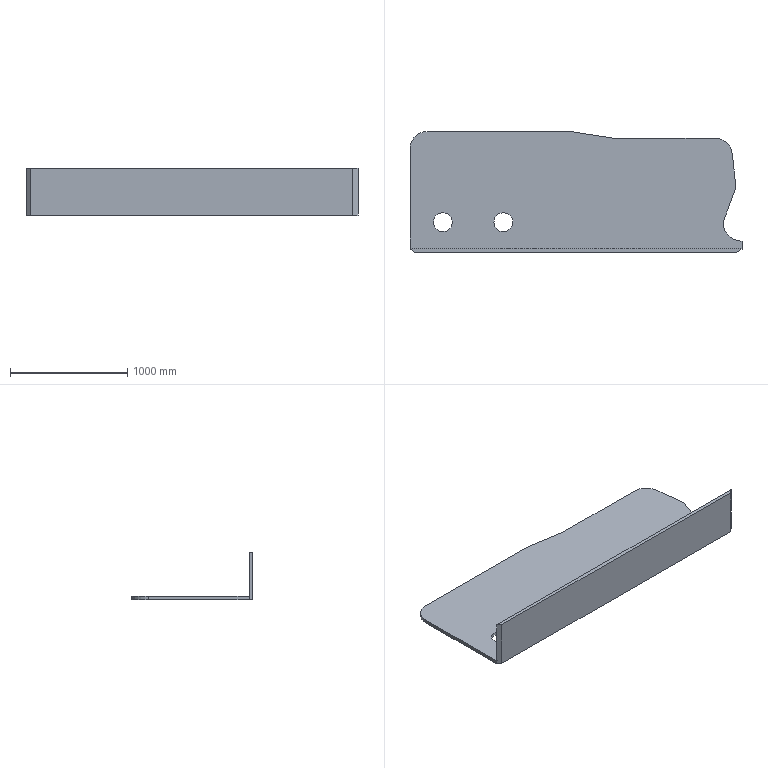Part | NX | features 掩护梁侧护板右 2 | 1 solid | 24 faces | box 2828 x 1030 x 405 mm | volume 109386503 mm3 | plane 18 | cylinder 6 | commonest cylinder face diameters 160.33 x2 291.509 x2 250.37 x1 322.604 x1
STEP:
#1=CARTESIAN_POINT('',(-541.636,-260.046,-750.));
#2=VERTEX_POINT('',#1);
#3=CARTESIAN_POINT('',(-621.801,-260.046,-750.));
#4=DIRECTION('',(0.,0.,1.));
#5=DIRECTION('',(1.,0.,0.));
#6=AXIS2_PLACEMENT_3D('',#3,#4,#5);
#7=CIRCLE('',#6,80.165);
#8=EDGE_CURVE('',#2,#2,#7,.T.);
#9=ORIENTED_EDGE('',*,*,#8,.F.);
#10=EDGE_LOOP('',(#9));
#11=FACE_BOUND('',#10,.T.);
#12=CARTESIAN_POINT('',(-1056.636,-260.046,-750.));
#13=VERTEX_POINT('',#12);
#14=CARTESIAN_POINT('',(-1136.801,-260.046,-750.));
#15=DIRECTION('',(0.,0.,1.));
#16=DIRECTION('',(1.,0.,0.));
#17=AXIS2_PLACEMENT_3D('',#14,#15,#16);
#18=CIRCLE('',#17,80.165);
#19=EDGE_CURVE('',#13,#13,#18,.T.);
#20=ORIENTED_EDGE('',*,*,#19,.F.);
#21=EDGE_LOOP('',(#20));
#22=FACE_BOUND('',#21,.T.);
#23=CARTESIAN_POINT('',(-1416.65,-488.395,-750.));
#24=VERTEX_POINT('',#23);
#25=CARTESIAN_POINT('',(1410.992,-488.395,-750.));
#26=VERTEX_POINT('',#25);
#27=CARTESIAN_POINT('',(1410.992,-488.395,-750.));
#28=DIRECTION('',(1.,0.,0.));
#29=VECTOR('',#28,1000.);
#30=LINE('',#27,#29);
#31=EDGE_CURVE('',#24,#26,#30,.T.);
#32=ORIENTED_EDGE('',*,*,#31,.T.);
#33=CARTESIAN_POINT('',(1410.992,-421.348,-750.));
#34=VERTEX_POINT('',#33);
#35=CARTESIAN_POINT('',(1410.992,-488.395,-750.));
#36=DIRECTION('',(0.,1.,0.));
#37=VECTOR('',#36,1000.);
#38=LINE('',#35,#37);
#39=EDGE_CURVE('',#26,#34,#38,.T.);
#40=ORIENTED_EDGE('',*,*,#39,.T.);
#41=CARTESIAN_POINT('',(1249.69,-260.046,-750.));
#42=VERTEX_POINT('',#41);
#43=CARTESIAN_POINT('',(1410.992,-260.046,-750.));
#44=DIRECTION('',(0.,0.,-1.));
#45=DIRECTION('',(1.,0.,0.));
#46=AXIS2_PLACEMENT_3D('',#43,#44,#45);
#47=CIRCLE('',#46,161.302);
#48=EDGE_CURVE('',#34,#42,#47,.T.);
#49=ORIENTED_EDGE('',*,*,#48,.T.);
#50=CARTESIAN_POINT('',(1359.76,36.697,-750.));
#51=VERTEX_POINT('',#50);
#52=CARTESIAN_POINT('',(1249.69,-260.046,-750.));
#53=DIRECTION('',(0.3478,0.9376,0.));
#54=VECTOR('',#53,1000.);
#55=LINE('',#52,#54);
#56=EDGE_CURVE('',#42,#51,#55,.T.);
#57=ORIENTED_EDGE('',*,*,#56,.T.);
#58=CARTESIAN_POINT('',(1327.809,324.481,-750.));
#59=VERTEX_POINT('',#58);
#60=CARTESIAN_POINT('',(1359.76,36.697,-750.));
#61=DIRECTION('',(-0.1103,0.9939,0.));
#62=VECTOR('',#61,1000.);
#63=LINE('',#60,#62);
#64=EDGE_CURVE('',#51,#59,#63,.T.);
#65=ORIENTED_EDGE('',*,*,#64,.T.);
#66=CARTESIAN_POINT('',(1182.944,454.152,-750.));
#67=VERTEX_POINT('',#66);
#68=CARTESIAN_POINT('',(1182.944,308.397,-750.));
#69=DIRECTION('',(0.,0.,1.));
#70=DIRECTION('',(1.,0.,0.));
#71=AXIS2_PLACEMENT_3D('',#68,#69,#70);
#72=CIRCLE('',#71,145.755);
#73=EDGE_CURVE('',#59,#67,#72,.T.);
#74=ORIENTED_EDGE('',*,*,#73,.T.);
#75=CARTESIAN_POINT('',(324.663,454.152,-750.));
#76=VERTEX_POINT('',#75);
#77=CARTESIAN_POINT('',(935.041,454.152,-750.));
#78=DIRECTION('',(-1.,0.,0.));
#79=VECTOR('',#78,1000.);
#80=LINE('',#77,#79);
#81=EDGE_CURVE('',#67,#76,#80,.T.);
#82=ORIENTED_EDGE('',*,*,#81,.T.);
#83=CARTESIAN_POINT('',(-51.414,512.454,-750.));
#84=VERTEX_POINT('',#83);
#85=CARTESIAN_POINT('',(324.663,454.152,-750.));
#86=DIRECTION('',(-0.9882,0.1532,0.));
#87=VECTOR('',#86,1000.);
#88=LINE('',#85,#87);
#89=EDGE_CURVE('',#76,#84,#88,.T.);
#90=ORIENTED_EDGE('',*,*,#89,.T.);
#91=CARTESIAN_POINT('',(-1270.895,512.454,-750.));
#92=VERTEX_POINT('',#91);
#93=CARTESIAN_POINT('',(-51.414,512.454,-750.));
#94=DIRECTION('',(-1.,0.,0.));
#95=VECTOR('',#94,1000.);
#96=LINE('',#93,#95);
#97=EDGE_CURVE('',#84,#92,#96,.T.);
#98=ORIENTED_EDGE('',*,*,#97,.T.);
#99=CARTESIAN_POINT('',(-1416.65,366.699,-750.));
#100=VERTEX_POINT('',#99);
#101=CARTESIAN_POINT('',(-1270.895,366.699,-750.));
#102=DIRECTION('',(0.,0.,1.));
#103=DIRECTION('',(1.,0.,0.));
#104=AXIS2_PLACEMENT_3D('',#101,#102,#103);
#105=CIRCLE('',#104,145.755);
#106=EDGE_CURVE('',#92,#100,#105,.T.);
#107=ORIENTED_EDGE('',*,*,#106,.T.);
#108=CARTESIAN_POINT('',(-1416.65,366.699,-750.));
#109=DIRECTION('',(0.,-1.,0.));
#110=VECTOR('',#109,1000.);
#111=LINE('',#108,#110);
#112=EDGE_CURVE('',#100,#24,#111,.T.);
#113=ORIENTED_EDGE('',*,*,#112,.T.);
#114=EDGE_LOOP('',(#32,#40,#49,#57,#65,#74,#82,#90,#98,#107,#113));
#115=FACE_BOUND('',#114,.T.);
#116=CARTESIAN_POINT('',(-1270.895,366.699,-750.));
#117=DIRECTION('',(0.,0.,-1.));
#118=DIRECTION('',(1.,0.,0.));
#119=AXIS2_PLACEMENT_3D('',#116,#117,#118);
#120=PLANE('',#119);
#121=ADVANCED_FACE('',(#11,#22,#115),#120,.F.);
#122=CARTESIAN_POINT('',(1410.992,-488.395,-775.));
#123=VERTEX_POINT('',#122);
#124=CARTESIAN_POINT('',(1410.992,-421.348,-775.));
#125=VERTEX_POINT('',#124);
#126=CARTESIAN_POINT('',(1410.992,-488.395,-775.));
#127=DIRECTION('',(0.,1.,0.));
#128=VECTOR('',#127,1000.);
#129=LINE('',#126,#128);
#130=EDGE_CURVE('',#123,#125,#129,.T.);
#131=ORIENTED_EDGE('',*,*,#130,.T.);
#132=CARTESIAN_POINT('',(1410.992,-421.348,-780.));
#133=DIRECTION('',(0.,0.,1.));
#134=VECTOR('',#133,1000.);
#135=LINE('',#132,#134);
#136=EDGE_CURVE('',#125,#34,#135,.T.);
#137=ORIENTED_EDGE('',*,*,#136,.T.);
#138=ORIENTED_EDGE('',*,*,#39,.F.);
#139=CARTESIAN_POINT('',(1410.992,-488.395,-780.));
#140=DIRECTION('',(0.,0.,1.));
#141=VECTOR('',#140,1000.);
#142=LINE('',#139,#141);
#143=EDGE_CURVE('',#123,#26,#142,.T.);
#144=ORIENTED_EDGE('',*,*,#143,.F.);
#145=EDGE_LOOP('',(#131,#137,#138,#144));
#146=FACE_BOUND('',#145,.T.);
#147=CARTESIAN_POINT('',(1410.992,-488.395,-780.));
#148=DIRECTION('',(-1.,0.,0.));
#149=DIRECTION('',(0.,-1.,0.));
#150=AXIS2_PLACEMENT_3D('',#147,#148,#149);
#151=PLANE('',#150);
#152=ADVANCED_FACE('',(#146),#151,.F.);
#153=CARTESIAN_POINT('',(1249.69,-260.046,-775.));
#154=VERTEX_POINT('',#153);
#155=CARTESIAN_POINT('',(1410.992,-260.046,-775.));
#156=DIRECTION('',(0.,0.,-1.));
#157=DIRECTION('',(1.,0.,0.));
#158=AXIS2_PLACEMENT_3D('',#155,#156,#157);
#159=CIRCLE('',#158,161.302);
#160=EDGE_CURVE('',#125,#154,#159,.T.);
#161=ORIENTED_EDGE('',*,*,#160,.T.);
#162=CARTESIAN_POINT('',(1249.69,-260.046,-780.));
#163=DIRECTION('',(0.,0.,1.));
#164=VECTOR('',#163,1000.);
#165=LINE('',#162,#164);
#166=EDGE_CURVE('',#154,#42,#165,.T.);
#167=ORIENTED_EDGE('',*,*,#166,.T.);
#168=ORIENTED_EDGE('',*,*,#48,.F.);
#169=ORIENTED_EDGE('',*,*,#136,.F.);
#170=EDGE_LOOP('',(#161,#167,#168,#169));
#171=FACE_BOUND('',#170,.T.);
#172=CARTESIAN_POINT('',(1410.992,-260.046,-780.));
#173=DIRECTION('',(0.,0.,1.));
#174=DIRECTION('',(-1.,0.,0.));
#175=AXIS2_PLACEMENT_3D('',#172,#173,#174);
#176=CYLINDRICAL_SURFACE('',#175,161.302);
#177=ADVANCED_FACE('',(#171),#176,.F.);
#178=CARTESIAN_POINT('',(1359.76,36.697,-775.));
#179=VERTEX_POINT('',#178);
#180=CARTESIAN_POINT('',(1249.69,-260.046,-775.));
#181=DIRECTION('',(0.3478,0.9376,0.));
#182=VECTOR('',#181,1000.);
#183=LINE('',#180,#182);
#184=EDGE_CURVE('',#154,#179,#183,.T.);
#185=ORIENTED_EDGE('',*,*,#184,.T.);
#186=CARTESIAN_POINT('',(1359.76,36.697,-780.));
#187=DIRECTION('',(0.,0.,1.));
#188=VECTOR('',#187,1000.);
#189=LINE('',#186,#188);
#190=EDGE_CURVE('',#179,#51,#189,.T.);
#191=ORIENTED_EDGE('',*,*,#190,.T.);
#192=ORIENTED_EDGE('',*,*,#56,.F.);
#193=ORIENTED_EDGE('',*,*,#166,.F.);
#194=EDGE_LOOP('',(#185,#191,#192,#193));
#195=FACE_BOUND('',#194,.T.);
#196=CARTESIAN_POINT('',(1249.69,-260.046,-780.));
#197=DIRECTION('',(-0.9376,0.3478,0.));
#198=DIRECTION('',(-0.3478,-0.9376,0.));
#199=AXIS2_PLACEMENT_3D('',#196,#197,#198);
#200=PLANE('',#199);
#201=ADVANCED_FACE('',(#195),#200,.F.);
#202=CARTESIAN_POINT('',(1327.809,324.481,-775.));
#203=VERTEX_POINT('',#202);
#204=CARTESIAN_POINT('',(1359.76,36.697,-775.));
#205=DIRECTION('',(-0.1103,0.9939,0.));
#206=VECTOR('',#205,1000.);
#207=LINE('',#204,#206);
#208=EDGE_CURVE('',#179,#203,#207,.T.);
#209=ORIENTED_EDGE('',*,*,#208,.T.);
#210=CARTESIAN_POINT('',(1327.809,324.481,-780.));
#211=DIRECTION('',(0.,0.,1.));
#212=VECTOR('',#211,1000.);
#213=LINE('',#210,#212);
#214=EDGE_CURVE('',#203,#59,#213,.T.);
#215=ORIENTED_EDGE('',*,*,#214,.T.);
#216=ORIENTED_EDGE('',*,*,#64,.F.);
#217=ORIENTED_EDGE('',*,*,#190,.F.);
#218=EDGE_LOOP('',(#209,#215,#216,#217));
#219=FACE_BOUND('',#218,.T.);
#220=CARTESIAN_POINT('',(1359.76,36.697,-780.));
#221=DIRECTION('',(-0.9939,-0.1103,0.));
#222=DIRECTION('',(0.1103,-0.9939,0.));
#223=AXIS2_PLACEMENT_3D('',#220,#221,#222);
#224=PLANE('',#223);
#225=ADVANCED_FACE('',(#219),#224,.F.);
#226=CARTESIAN_POINT('',(1182.944,454.152,-775.));
#227=VERTEX_POINT('',#226);
#228=CARTESIAN_POINT('',(1182.944,308.397,-775.));
#229=DIRECTION('',(0.,0.,1.));
#230=DIRECTION('',(1.,0.,0.));
#231=AXIS2_PLACEMENT_3D('',#228,#229,#230);
#232=CIRCLE('',#231,145.755);
#233=EDGE_CURVE('',#203,#227,#232,.T.);
#234=ORIENTED_EDGE('',*,*,#233,.T.);
#235=CARTESIAN_POINT('',(1182.944,454.152,-780.));
#236=DIRECTION('',(0.,0.,1.));
#237=VECTOR('',#236,1000.);
#238=LINE('',#235,#237);
#239=EDGE_CURVE('',#227,#67,#238,.T.);
#240=ORIENTED_EDGE('',*,*,#239,.T.);
#241=ORIENTED_EDGE('',*,*,#73,.F.);
#242=ORIENTED_EDGE('',*,*,#214,.F.);
#243=EDGE_LOOP('',(#234,#240,#241,#242));
#244=FACE_BOUND('',#243,.T.);
#245=CARTESIAN_POINT('',(1182.944,308.397,-780.));
#246=DIRECTION('',(0.,0.,1.));
#247=DIRECTION('',(-1.,0.,0.));
#248=AXIS2_PLACEMENT_3D('',#245,#246,#247);
#249=CYLINDRICAL_SURFACE('',#248,145.755);
#250=ADVANCED_FACE('',(#244),#249,.T.);
#251=CARTESIAN_POINT('',(1337.166,-488.395,-780.));
#252=VERTEX_POINT('',#251);
#253=CARTESIAN_POINT('',(1410.992,-488.395,-780.));
#254=VERTEX_POINT('',#253);
#255=CARTESIAN_POINT('',(1337.166,-488.395,-780.));
#256=DIRECTION('',(1.,0.,0.));
#257=VECTOR('',#256,1000.);
#258=LINE('',#255,#257);
#259=EDGE_CURVE('',#252,#254,#258,.T.);
#260=ORIENTED_EDGE('',*,*,#259,.T.);
#261=CARTESIAN_POINT('',(1367.913,-517.546,-780.));
#262=VERTEX_POINT('',#261);
#263=CARTESIAN_POINT('',(1410.992,-488.395,-780.));
#264=DIRECTION('',(0.8282,0.5604,0.));
#265=VECTOR('',#264,1000.);
#266=LINE('',#263,#265);
#267=EDGE_CURVE('',#262,#254,#266,.T.);
#268=ORIENTED_EDGE('',*,*,#267,.F.);
#269=CARTESIAN_POINT('',(-1381.422,-517.546,-780.));
#270=VERTEX_POINT('',#269);
#271=CARTESIAN_POINT('',(1367.913,-517.546,-780.));
#272=DIRECTION('',(1.,0.,0.));
#273=VECTOR('',#272,1000.);
#274=LINE('',#271,#273);
#275=EDGE_CURVE('',#270,#262,#274,.T.);
#276=ORIENTED_EDGE('',*,*,#275,.F.);
#277=CARTESIAN_POINT('',(-1416.65,-488.395,-780.));
#278=VERTEX_POINT('',#277);
#279=CARTESIAN_POINT('',(-1381.422,-517.546,-780.));
#280=DIRECTION('',(0.7704,-0.6375,0.));
#281=VECTOR('',#280,1000.);
#282=LINE('',#279,#281);
#283=EDGE_CURVE('',#278,#270,#282,.T.);
#284=ORIENTED_EDGE('',*,*,#283,.F.);
#285=CARTESIAN_POINT('',(-1416.65,366.699,-780.));
#286=VERTEX_POINT('',#285);
#287=CARTESIAN_POINT('',(-1416.65,366.699,-780.));
#288=DIRECTION('',(0.,-1.,0.));
#289=VECTOR('',#288,1000.);
#290=LINE('',#287,#289);
#291=EDGE_CURVE('',#286,#278,#290,.T.);
#292=ORIENTED_EDGE('',*,*,#291,.F.);
#293=CARTESIAN_POINT('',(-1270.895,512.454,-780.));
#294=VERTEX_POINT('',#293);
#295=CARTESIAN_POINT('',(-1270.895,366.699,-780.));
#296=DIRECTION('',(0.,0.,1.));
#297=DIRECTION('',(1.,0.,0.));
#298=AXIS2_PLACEMENT_3D('',#295,#296,#297);
#299=CIRCLE('',#298,145.755);
#300=EDGE_CURVE('',#294,#286,#299,.T.);
#301=ORIENTED_EDGE('',*,*,#300,.F.);
#302=CARTESIAN_POINT('',(-51.414,512.454,-780.));
#303=VERTEX_POINT('',#302);
#304=CARTESIAN_POINT('',(-51.414,512.454,-780.));
#305=DIRECTION('',(-1.,0.,0.));
#306=VECTOR('',#305,1000.);
#307=LINE('',#304,#306);
#308=EDGE_CURVE('',#303,#294,#307,.T.);
#309=ORIENTED_EDGE('',*,*,#308,.F.);
#310=CARTESIAN_POINT('',(324.663,454.152,-780.));
#311=VERTEX_POINT('',#310);
#312=CARTESIAN_POINT('',(324.663,454.152,-780.));
#313=DIRECTION('',(-0.9882,0.1532,0.));
#314=VECTOR('',#313,1000.);
#315=LINE('',#312,#314);
#316=EDGE_CURVE('',#311,#303,#315,.T.);
#317=ORIENTED_EDGE('',*,*,#316,.F.);
#318=CARTESIAN_POINT('',(935.041,454.152,-780.));
#319=VERTEX_POINT('',#318);
#320=CARTESIAN_POINT('',(1182.944,454.152,-780.));
#321=DIRECTION('',(-1.,0.,0.));
#322=VECTOR('',#321,1000.);
#323=LINE('',#320,#322);
#324=EDGE_CURVE('',#319,#311,#323,.T.);
#325=ORIENTED_EDGE('',*,*,#324,.F.);
#326=CARTESIAN_POINT('',(688.438,-132.458,-780.));
#327=VERTEX_POINT('',#326);
#328=CARTESIAN_POINT('',(935.041,454.152,-780.));
#329=DIRECTION('',(-0.3875,-0.9219,0.));
#330=VECTOR('',#329,1000.);
#331=LINE('',#328,#330);
#332=EDGE_CURVE('',#319,#327,#331,.T.);
#333=ORIENTED_EDGE('',*,*,#332,.T.);
#334=CARTESIAN_POINT('',(764.685,-299.875,-780.));
#335=VERTEX_POINT('',#334);
#336=CARTESIAN_POINT('',(803.841,-180.971,-780.));
#337=DIRECTION('',(0.,0.,1.));
#338=DIRECTION('',(1.,0.,0.));
#339=AXIS2_PLACEMENT_3D('',#336,#337,#338);
#340=CIRCLE('',#339,125.185);
#341=EDGE_CURVE('',#327,#335,#340,.T.);
#342=ORIENTED_EDGE('',*,*,#341,.T.);
#343=CARTESIAN_POINT('',(764.685,-299.875,-780.));
#344=DIRECTION('',(0.9498,-0.3128,0.));
#345=VECTOR('',#344,1000.);
#346=LINE('',#343,#345);
#347=EDGE_CURVE('',#335,#252,#346,.T.);
#348=ORIENTED_EDGE('',*,*,#347,.T.);
#349=EDGE_LOOP('',(#260,#268,#276,#284,#292,#301,#309,#317,#325,#333,#342,#348));
#350=FACE_BOUND('',#349,.T.);
#351=CARTESIAN_POINT('',(-1056.636,-260.046,-780.));
#352=VERTEX_POINT('',#351);
#353=CARTESIAN_POINT('',(-1136.801,-260.046,-780.));
#354=DIRECTION('',(0.,0.,1.));
#355=DIRECTION('',(1.,0.,0.));
#356=AXIS2_PLACEMENT_3D('',#353,#354,#355);
#357=CIRCLE('',#356,80.165);
#358=EDGE_CURVE('',#352,#352,#357,.T.);
#359=ORIENTED_EDGE('',*,*,#358,.T.);
#360=EDGE_LOOP('',(#359));
#361=FACE_BOUND('',#360,.T.);
#362=CARTESIAN_POINT('',(-541.636,-260.046,-780.));
#363=VERTEX_POINT('',#362);
#364=CARTESIAN_POINT('',(-621.801,-260.046,-780.));
#365=DIRECTION('',(0.,0.,1.));
#366=DIRECTION('',(1.,0.,0.));
#367=AXIS2_PLACEMENT_3D('',#364,#365,#366);
#368=CIRCLE('',#367,80.165);
#369=EDGE_CURVE('',#363,#363,#368,.T.);
#370=ORIENTED_EDGE('',*,*,#369,.T.);
#371=EDGE_LOOP('',(#370));
#372=FACE_BOUND('',#371,.T.);
#373=CARTESIAN_POINT('',(-1270.895,366.699,-780.));
#374=DIRECTION('',(0.,0.,-1.));
#375=DIRECTION('',(1.,0.,0.));
#376=AXIS2_PLACEMENT_3D('',#373,#374,#375);
#377=PLANE('',#376);
#378=ADVANCED_FACE('',(#350,#361,#372),#377,.T.);
#379=ORIENTED_EDGE('',*,*,#106,.F.);
#380=CARTESIAN_POINT('',(-1270.895,512.454,-780.));
#381=DIRECTION('',(0.,0.,1.));
#382=VECTOR('',#381,1000.);
#383=LINE('',#380,#382);
#384=EDGE_CURVE('',#294,#92,#383,.T.);
#385=ORIENTED_EDGE('',*,*,#384,.F.);
#386=ORIENTED_EDGE('',*,*,#300,.T.);
#387=CARTESIAN_POINT('',(-1416.65,366.699,-780.));
#388=DIRECTION('',(0.,0.,1.));
#389=VECTOR('',#388,1000.);
#390=LINE('',#387,#389);
#391=EDGE_CURVE('',#286,#100,#390,.T.);
#392=ORIENTED_EDGE('',*,*,#391,.T.);
#393=EDGE_LOOP('',(#379,#385,#386,#392));
#394=FACE_BOUND('',#393,.T.);
#395=CARTESIAN_POINT('',(-1270.895,366.699,-780.));
#396=DIRECTION('',(0.,0.,1.));
#397=DIRECTION('',(-1.,0.,0.));
#398=AXIS2_PLACEMENT_3D('',#395,#396,#397);
#399=CYLINDRICAL_SURFACE('',#398,145.755);
#400=ADVANCED_FACE('',(#394),#399,.T.);
#401=ORIENTED_EDGE('',*,*,#112,.F.);
#402=ORIENTED_EDGE('',*,*,#391,.F.);
#403=ORIENTED_EDGE('',*,*,#291,.T.);
#404=CARTESIAN_POINT('',(-1416.65,-488.395,-780.));
#405=DIRECTION('',(0.,0.,1.));
#406=VECTOR('',#405,1000.);
#407=LINE('',#404,#406);
#408=EDGE_CURVE('',#278,#24,#407,.T.);
#409=ORIENTED_EDGE('',*,*,#408,.T.);
#410=EDGE_LOOP('',(#401,#402,#403,#409));
#411=FACE_BOUND('',#410,.T.);
#412=CARTESIAN_POINT('',(-1416.65,366.699,-780.));
#413=DIRECTION('',(1.,0.,0.));
#414=DIRECTION('',(0.,0.,1.));
#415=AXIS2_PLACEMENT_3D('',#412,#413,#414);
#416=PLANE('',#415);
#417=ADVANCED_FACE('',(#411),#416,.F.);
#418=ORIENTED_EDGE('',*,*,#408,.F.);
#419=ORIENTED_EDGE('',*,*,#283,.T.);
#420=CARTESIAN_POINT('',(-1381.422,-517.546,-375.));
#421=VERTEX_POINT('',#420);
#422=CARTESIAN_POINT('',(-1381.422,-517.546,-780.));
#423=DIRECTION('',(0.,0.,1.));
#424=VECTOR('',#423,1000.);
#425=LINE('',#422,#424);
#426=EDGE_CURVE('',#270,#421,#425,.T.);
#427=ORIENTED_EDGE('',*,*,#426,.T.);
#428=CARTESIAN_POINT('',(-1416.65,-488.395,-375.));
#429=VERTEX_POINT('',#428);
#430=CARTESIAN_POINT('',(-1416.65,-488.395,-375.));
#431=DIRECTION('',(-0.7704,0.6375,0.));
#432=VECTOR('',#431,1000.);
#433=LINE('',#430,#432);
#434=EDGE_CURVE('',#421,#429,#433,.T.);
#435=ORIENTED_EDGE('',*,*,#434,.T.);
#436=CARTESIAN_POINT('',(-1416.65,-488.395,-375.));
#437=DIRECTION('',(0.,0.,-1.));
#438=VECTOR('',#437,1000.);
#439=LINE('',#436,#438);
#440=EDGE_CURVE('',#429,#24,#439,.T.);
#441=ORIENTED_EDGE('',*,*,#440,.T.);
#442=EDGE_LOOP('',(#418,#419,#427,#435,#441));
#443=FACE_BOUND('',#442,.T.);
#444=CARTESIAN_POINT('',(-1381.422,-517.546,-780.));
#445=DIRECTION('',(0.6375,0.7704,0.));
#446=DIRECTION('',(-0.7704,0.6375,0.));
#447=AXIS2_PLACEMENT_3D('',#444,#445,#446);
#448=PLANE('',#447);
#449=ADVANCED_FACE('',(#443),#448,.F.);
#450=ORIENTED_EDGE('',*,*,#426,.F.);
#451=ORIENTED_EDGE('',*,*,#275,.T.);
#452=CARTESIAN_POINT('',(1367.913,-517.546,-375.));
#453=VERTEX_POINT('',#452);
#454=CARTESIAN_POINT('',(1367.913,-517.546,-780.));
#455=DIRECTION('',(0.,0.,1.));
#456=VECTOR('',#455,1000.);
#457=LINE('',#454,#456);
#458=EDGE_CURVE('',#262,#453,#457,.T.);
#459=ORIENTED_EDGE('',*,*,#458,.T.);
#460=CARTESIAN_POINT('',(-1381.422,-517.546,-375.));
#461=DIRECTION('',(-1.,0.,0.));
#462=VECTOR('',#461,1000.);
#463=LINE('',#460,#462);
#464=EDGE_CURVE('',#453,#421,#463,.T.);
#465=ORIENTED_EDGE('',*,*,#464,.T.);
#466=EDGE_LOOP('',(#450,#451,#459,#465));
#467=FACE_BOUND('',#466,.T.);
#468=CARTESIAN_POINT('',(1367.913,-517.546,-780.));
#469=DIRECTION('',(0.,1.,0.));
#470=DIRECTION('',(-1.,0.,0.));
#471=AXIS2_PLACEMENT_3D('',#468,#469,#470);
#472=PLANE('',#471);
#473=ADVANCED_FACE('',(#467),#472,.F.);
#474=ORIENTED_EDGE('',*,*,#458,.F.);
#475=ORIENTED_EDGE('',*,*,#267,.T.);
#476=CARTESIAN_POINT('',(1410.992,-488.395,-780.));
#477=DIRECTION('',(0.,0.,1.));
#478=VECTOR('',#477,1000.);
#479=LINE('',#476,#478);
#480=EDGE_CURVE('',#254,#123,#479,.T.);
#481=ORIENTED_EDGE('',*,*,#480,.T.);
#482=ORIENTED_EDGE('',*,*,#143,.T.);
#483=CARTESIAN_POINT('',(1410.992,-488.395,-375.));
#484=VERTEX_POINT('',#483);
#485=CARTESIAN_POINT('',(1410.992,-488.395,-375.));
#486=DIRECTION('',(0.,0.,-1.));
#487=VECTOR('',#486,1000.);
#488=LINE('',#485,#487);
#489=EDGE_CURVE('',#484,#26,#488,.T.);
#490=ORIENTED_EDGE('',*,*,#489,.F.);
#491=CARTESIAN_POINT('',(1367.913,-517.546,-375.));
#492=DIRECTION('',(-0.8282,-0.5604,0.));
#493=VECTOR('',#492,1000.);
#494=LINE('',#491,#493);
#495=EDGE_CURVE('',#484,#453,#494,.T.);
#496=ORIENTED_EDGE('',*,*,#495,.T.);
#497=EDGE_LOOP('',(#474,#475,#481,#482,#490,#496));
#498=FACE_BOUND('',#497,.T.);
#499=CARTESIAN_POINT('',(1410.992,-488.395,-780.));
#500=DIRECTION('',(-0.5604,0.8282,0.));
#501=DIRECTION('',(-0.8282,-0.5604,0.));
#502=AXIS2_PLACEMENT_3D('',#499,#500,#501);
#503=PLANE('',#502);
#504=ADVANCED_FACE('',(#498),#503,.F.);
#505=ORIENTED_EDGE('',*,*,#324,.T.);
#506=CARTESIAN_POINT('',(324.663,454.152,-780.));
#507=DIRECTION('',(0.,0.,1.));
#508=VECTOR('',#507,1000.);
#509=LINE('',#506,#508);
#510=EDGE_CURVE('',#311,#76,#509,.T.);
#511=ORIENTED_EDGE('',*,*,#510,.T.);
#512=ORIENTED_EDGE('',*,*,#81,.F.);
#513=ORIENTED_EDGE('',*,*,#239,.F.);
#514=CARTESIAN_POINT('',(935.041,454.152,-775.));
#515=VERTEX_POINT('',#514);
#516=CARTESIAN_POINT('',(935.041,454.152,-775.));
#517=DIRECTION('',(-1.,0.,0.));
#518=VECTOR('',#517,1000.);
#519=LINE('',#516,#518);
#520=EDGE_CURVE('',#227,#515,#519,.T.);
#521=ORIENTED_EDGE('',*,*,#520,.T.);
#522=CARTESIAN_POINT('',(935.041,454.152,-775.));
#523=DIRECTION('',(0.,0.,-1.));
#524=VECTOR('',#523,1000.);
#525=LINE('',#522,#524);
#526=EDGE_CURVE('',#515,#319,#525,.T.);
#527=ORIENTED_EDGE('',*,*,#526,.T.);
#528=EDGE_LOOP('',(#505,#511,#512,#513,#521,#527));
#529=FACE_BOUND('',#528,.T.);
#530=CARTESIAN_POINT('',(935.041,454.152,-780.));
#531=DIRECTION('',(0.,-1.,0.));
#532=DIRECTION('',(1.,0.,0.));
#533=AXIS2_PLACEMENT_3D('',#530,#531,#532);
#534=PLANE('',#533);
#535=ADVANCED_FACE('',(#529),#534,.F.);
#536=ORIENTED_EDGE('',*,*,#89,.F.);
#537=ORIENTED_EDGE('',*,*,#510,.F.);
#538=ORIENTED_EDGE('',*,*,#316,.T.);
#539=CARTESIAN_POINT('',(-51.414,512.454,-780.));
#540=DIRECTION('',(0.,0.,1.));
#541=VECTOR('',#540,1000.);
#542=LINE('',#539,#541);
#543=EDGE_CURVE('',#303,#84,#542,.T.);
#544=ORIENTED_EDGE('',*,*,#543,.T.);
#545=EDGE_LOOP('',(#536,#537,#538,#544));
#546=FACE_BOUND('',#545,.T.);
#547=CARTESIAN_POINT('',(324.663,454.152,-780.));
#548=DIRECTION('',(-0.1532,-0.9882,0.));
#549=DIRECTION('',(0.9882,-0.1532,0.));
#550=AXIS2_PLACEMENT_3D('',#547,#548,#549);
#551=PLANE('',#550);
#552=ADVANCED_FACE('',(#546),#551,.F.);
#553=ORIENTED_EDGE('',*,*,#97,.F.);
#554=ORIENTED_EDGE('',*,*,#543,.F.);
#555=ORIENTED_EDGE('',*,*,#308,.T.);
#556=ORIENTED_EDGE('',*,*,#384,.T.);
#557=EDGE_LOOP('',(#553,#554,#555,#556));
#558=FACE_BOUND('',#557,.T.);
#559=CARTESIAN_POINT('',(-51.414,512.454,-780.));
#560=DIRECTION('',(0.,-1.,0.));
#561=DIRECTION('',(0.,0.,1.));
#562=AXIS2_PLACEMENT_3D('',#559,#560,#561);
#563=PLANE('',#562);
#564=ADVANCED_FACE('',(#558),#563,.F.);
#565=ORIENTED_EDGE('',*,*,#358,.F.);
#566=EDGE_LOOP('',(#565));
#567=FACE_BOUND('',#566,.T.);
#568=ORIENTED_EDGE('',*,*,#19,.T.);
#569=EDGE_LOOP('',(#568));
#570=FACE_BOUND('',#569,.T.);
#571=CARTESIAN_POINT('',(-1136.801,-260.046,-780.));
#572=DIRECTION('',(0.,0.,1.));
#573=DIRECTION('',(-1.,0.,0.));
#574=AXIS2_PLACEMENT_3D('',#571,#572,#573);
#575=CYLINDRICAL_SURFACE('',#574,80.165);
#576=ADVANCED_FACE('',(#567,#570),#575,.F.);
#577=ORIENTED_EDGE('',*,*,#369,.F.);
#578=EDGE_LOOP('',(#577));
#579=FACE_BOUND('',#578,.T.);
#580=ORIENTED_EDGE('',*,*,#8,.T.);
#581=EDGE_LOOP('',(#580));
#582=FACE_BOUND('',#581,.T.);
#583=CARTESIAN_POINT('',(-621.801,-260.046,-780.));
#584=DIRECTION('',(0.,0.,1.));
#585=DIRECTION('',(-1.,0.,0.));
#586=AXIS2_PLACEMENT_3D('',#583,#584,#585);
#587=CYLINDRICAL_SURFACE('',#586,80.165);
#588=ADVANCED_FACE('',(#579,#582),#587,.F.);
#589=ORIENTED_EDGE('',*,*,#259,.F.);
#590=CARTESIAN_POINT('',(1337.166,-488.395,-775.));
#591=VERTEX_POINT('',#590);
#592=CARTESIAN_POINT('',(1337.166,-488.395,-775.));
#593=DIRECTION('',(0.,0.,-1.));
#594=VECTOR('',#593,1000.);
#595=LINE('',#592,#594);
#596=EDGE_CURVE('',#591,#252,#595,.T.);
#597=ORIENTED_EDGE('',*,*,#596,.F.);
#598=CARTESIAN_POINT('',(1337.166,-488.395,-775.));
#599=DIRECTION('',(1.,0.,0.));
#600=VECTOR('',#599,1000.);
#601=LINE('',#598,#600);
#602=EDGE_CURVE('',#591,#123,#601,.T.);
#603=ORIENTED_EDGE('',*,*,#602,.T.);
#604=ORIENTED_EDGE('',*,*,#480,.F.);
#605=EDGE_LOOP('',(#589,#597,#603,#604));
#606=FACE_BOUND('',#605,.T.);
#607=CARTESIAN_POINT('',(1337.166,-488.395,-775.));
#608=DIRECTION('',(0.,-1.,0.));
#609=DIRECTION('',(0.,0.,1.));
#610=AXIS2_PLACEMENT_3D('',#607,#608,#609);
#611=PLANE('',#610);
#612=ADVANCED_FACE('',(#606),#611,.F.);
#613=ORIENTED_EDGE('',*,*,#347,.F.);
#614=CARTESIAN_POINT('',(764.685,-299.875,-775.));
#615=VERTEX_POINT('',#614);
#616=CARTESIAN_POINT('',(764.685,-299.875,-775.));
#617=DIRECTION('',(0.,0.,-1.));
#618=VECTOR('',#617,1000.);
#619=LINE('',#616,#618);
#620=EDGE_CURVE('',#615,#335,#619,.T.);
#621=ORIENTED_EDGE('',*,*,#620,.F.);
#622=CARTESIAN_POINT('',(764.685,-299.875,-775.));
#623=DIRECTION('',(0.9498,-0.3128,0.));
#624=VECTOR('',#623,1000.);
#625=LINE('',#622,#624);
#626=EDGE_CURVE('',#615,#591,#625,.T.);
#627=ORIENTED_EDGE('',*,*,#626,.T.);
#628=ORIENTED_EDGE('',*,*,#596,.T.);
#629=EDGE_LOOP('',(#613,#621,#627,#628));
#630=FACE_BOUND('',#629,.T.);
#631=CARTESIAN_POINT('',(764.685,-299.875,-775.));
#632=DIRECTION('',(-0.3128,-0.9498,0.));
#633=DIRECTION('',(0.9498,-0.3128,0.));
#634=AXIS2_PLACEMENT_3D('',#631,#632,#633);
#635=PLANE('',#634);
#636=ADVANCED_FACE('',(#630),#635,.F.);
#637=ORIENTED_EDGE('',*,*,#341,.F.);
#638=CARTESIAN_POINT('',(688.438,-132.458,-775.));
#639=VERTEX_POINT('',#638);
#640=CARTESIAN_POINT('',(688.438,-132.458,-775.));
#641=DIRECTION('',(0.,0.,-1.));
#642=VECTOR('',#641,1000.);
#643=LINE('',#640,#642);
#644=EDGE_CURVE('',#639,#327,#643,.T.);
#645=ORIENTED_EDGE('',*,*,#644,.F.);
#646=CARTESIAN_POINT('',(803.841,-180.971,-775.));
#647=DIRECTION('',(0.,0.,1.));
#648=DIRECTION('',(1.,0.,0.));
#649=AXIS2_PLACEMENT_3D('',#646,#647,#648);
#650=CIRCLE('',#649,125.185);
#651=EDGE_CURVE('',#639,#615,#650,.T.);
#652=ORIENTED_EDGE('',*,*,#651,.T.);
#653=ORIENTED_EDGE('',*,*,#620,.T.);
#654=EDGE_LOOP('',(#637,#645,#652,#653));
#655=FACE_BOUND('',#654,.T.);
#656=CARTESIAN_POINT('',(803.841,-180.971,-775.));
#657=DIRECTION('',(0.,0.,-1.));
#658=DIRECTION('',(1.,0.,0.));
#659=AXIS2_PLACEMENT_3D('',#656,#657,#658);
#660=CYLINDRICAL_SURFACE('',#659,125.185);
#661=ADVANCED_FACE('',(#655),#660,.F.);
#662=ORIENTED_EDGE('',*,*,#332,.F.);
#663=ORIENTED_EDGE('',*,*,#526,.F.);
#664=CARTESIAN_POINT('',(935.041,454.152,-775.));
#665=DIRECTION('',(-0.3875,-0.9219,0.));
#666=VECTOR('',#665,1000.);
#667=LINE('',#664,#666);
#668=EDGE_CURVE('',#515,#639,#667,.T.);
#669=ORIENTED_EDGE('',*,*,#668,.T.);
#670=ORIENTED_EDGE('',*,*,#644,.T.);
#671=EDGE_LOOP('',(#662,#663,#669,#670));
#672=FACE_BOUND('',#671,.T.);
#673=CARTESIAN_POINT('',(935.041,454.152,-775.));
#674=DIRECTION('',(-0.9219,0.3875,0.));
#675=DIRECTION('',(-0.3875,-0.9219,0.));
#676=AXIS2_PLACEMENT_3D('',#673,#674,#675);
#677=PLANE('',#676);
#678=ADVANCED_FACE('',(#672),#677,.F.);
#679=ORIENTED_EDGE('',*,*,#520,.F.);
#680=ORIENTED_EDGE('',*,*,#233,.F.);
#681=ORIENTED_EDGE('',*,*,#208,.F.);
#682=ORIENTED_EDGE('',*,*,#184,.F.);
#683=ORIENTED_EDGE('',*,*,#160,.F.);
#684=ORIENTED_EDGE('',*,*,#130,.F.);
#685=ORIENTED_EDGE('',*,*,#602,.F.);
#686=ORIENTED_EDGE('',*,*,#626,.F.);
#687=ORIENTED_EDGE('',*,*,#651,.F.);
#688=ORIENTED_EDGE('',*,*,#668,.F.);
#689=EDGE_LOOP('',(#679,#680,#681,#682,#683,#684,#685,#686,#687,#688));
#690=FACE_BOUND('',#689,.T.);
#691=CARTESIAN_POINT('',(1182.944,308.397,-775.));
#692=DIRECTION('',(0.,0.,-1.));
#693=DIRECTION('',(1.,0.,0.));
#694=AXIS2_PLACEMENT_3D('',#691,#692,#693);
#695=PLANE('',#694);
#696=ADVANCED_FACE('',(#690),#695,.T.);
#697=ORIENTED_EDGE('',*,*,#31,.F.);
#698=ORIENTED_EDGE('',*,*,#440,.F.);
#699=CARTESIAN_POINT('',(1410.992,-488.395,-375.));
#700=DIRECTION('',(1.,0.,0.));
#701=VECTOR('',#700,1000.);
#702=LINE('',#699,#701);
#703=EDGE_CURVE('',#429,#484,#702,.T.);
#704=ORIENTED_EDGE('',*,*,#703,.T.);
#705=ORIENTED_EDGE('',*,*,#489,.T.);
#706=EDGE_LOOP('',(#697,#698,#704,#705));
#707=FACE_BOUND('',#706,.T.);
#708=CARTESIAN_POINT('',(1410.992,-488.395,-375.));
#709=DIRECTION('',(0.,-1.,0.));
#710=DIRECTION('',(0.,0.,1.));
#711=AXIS2_PLACEMENT_3D('',#708,#709,#710);
#712=PLANE('',#711);
#713=ADVANCED_FACE('',(#707),#712,.F.);
#714=ORIENTED_EDGE('',*,*,#495,.F.);
#715=ORIENTED_EDGE('',*,*,#703,.F.);
#716=ORIENTED_EDGE('',*,*,#434,.F.);
#717=ORIENTED_EDGE('',*,*,#464,.F.);
#718=EDGE_LOOP('',(#714,#715,#716,#717));
#719=FACE_BOUND('',#718,.T.);
#720=CARTESIAN_POINT('',(-144.576,-1541.031,-375.));
#721=DIRECTION('',(0.,0.,1.));
#722=DIRECTION('',(-1.,0.,0.));
#723=AXIS2_PLACEMENT_3D('',#720,#721,#722);
#724=PLANE('',#723);
#725=ADVANCED_FACE('',(#719),#724,.T.);
#726=CLOSED_SHELL('',(#121,#152,#177,#201,#225,#250,#378,#400,#417,#449,#473,#504,#535,#552,#564,#576,#588,#612,#636,#661,#678,#696,#713,#725));
#727=MANIFOLD_SOLID_BREP('',#726);
#728=(LENGTH_UNIT()NAMED_UNIT(*)SI_UNIT(.MILLI.,.METRE.));
#729=UNCERTAINTY_MEASURE_WITH_UNIT(LENGTH_MEASURE(0.00001),#728,'','');
#730=(NAMED_UNIT(*)PLANE_ANGLE_UNIT()SI_UNIT($,.RADIAN.));
#731=(NAMED_UNIT(*)SI_UNIT($,.STERADIAN.)SOLID_ANGLE_UNIT());
#732=(GEOMETRIC_REPRESENTATION_CONTEXT(3)GLOBAL_UNCERTAINTY_ASSIGNED_CONTEXT((#729))GLOBAL_UNIT_ASSIGNED_CONTEXT((#728,#730,#731))REPRESENTATION_CONTEXT('',''));
#733=ADVANCED_BREP_SHAPE_REPRESENTATION('',(#727),#732);